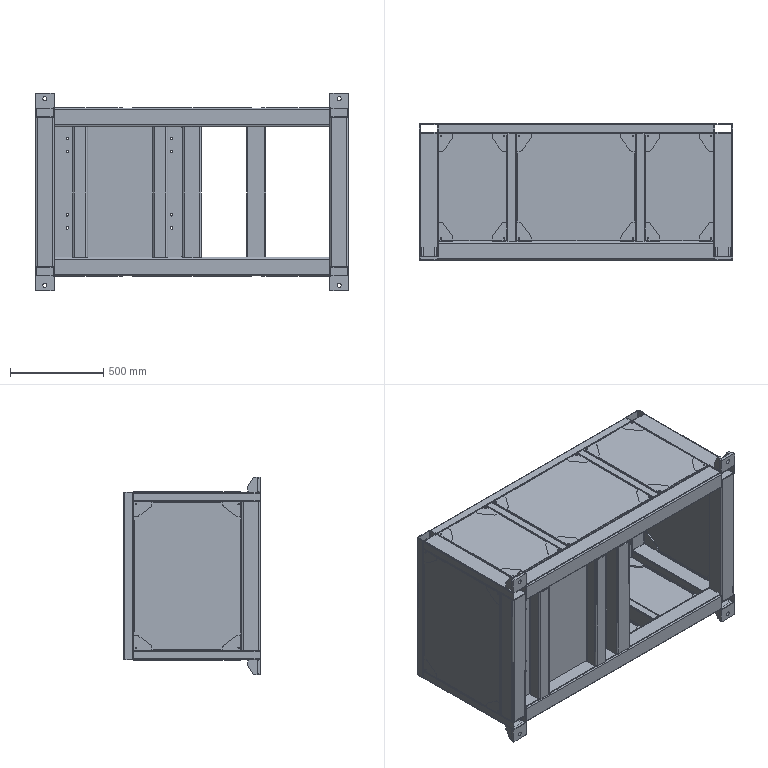Part | SolidWorks | 74 solids | 1582 faces | box 1682 x 730 x 1060 mm | volume 39110385 mm3 | plane 1054 | cylinder 528 | commonest cylinder face diameters 10 x174 40 x72 7 x64 2 x58 20 x40 1 x32